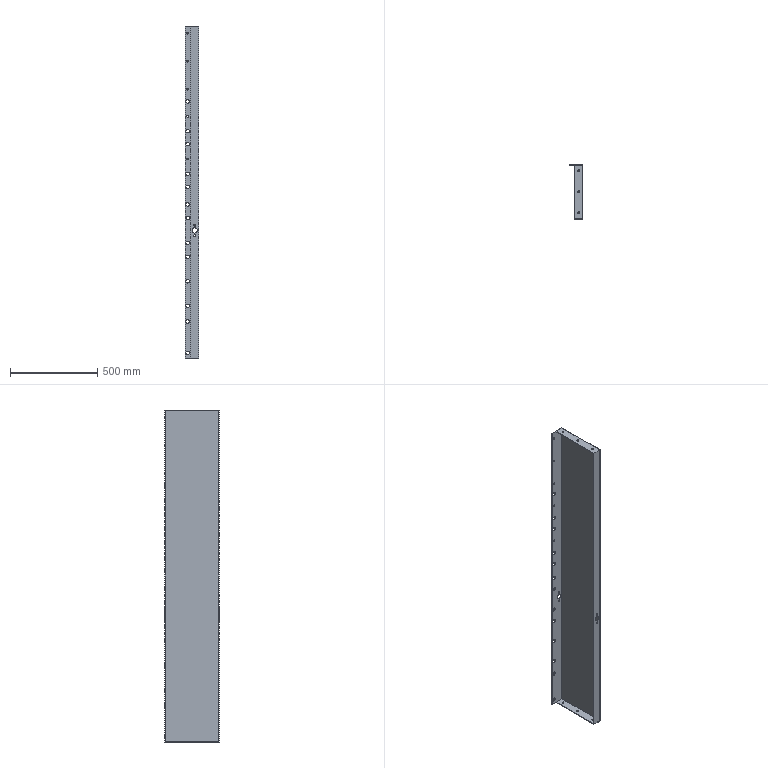Part | SolidWorks | features BaseBody 1 | 1 solid | 72 faces | box 80 x 310 x 1900 mm | volume 2538901 mm3 | cylinder 60 | plane 12 | commonest cylinder face diameters 20 x26 11 x16 10.6 x14 30 x4